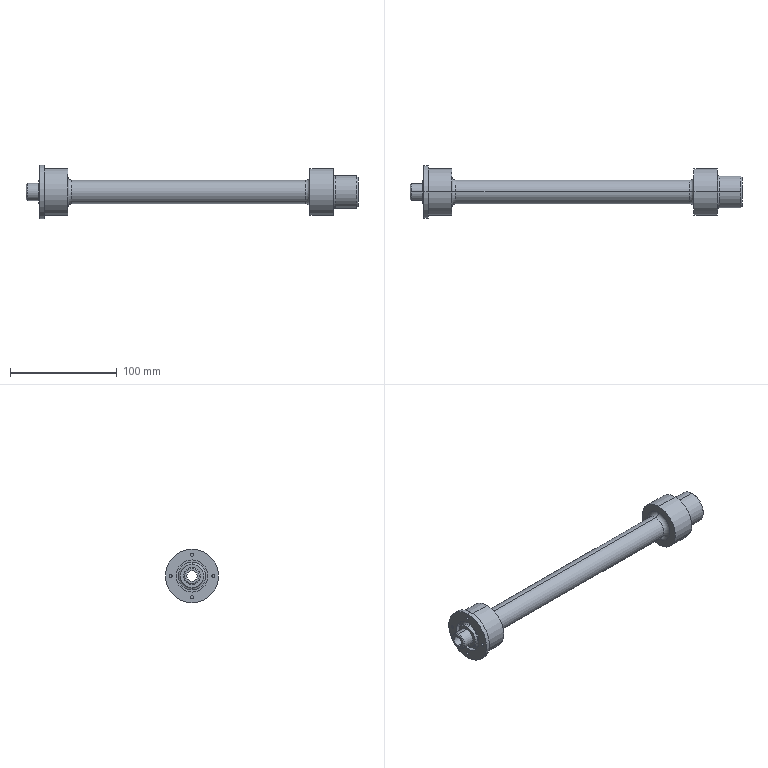Part | NX | features BREP 1 | 1 solid | 51 faces | box 311 x 50 x 50 mm | volume 154727 mm3 | cylinder 26 | plane 13 | torus 8 | cone 4 | commonest cylinder face diameters 3 x8 22 x4 30 x4 44 x4 10 x2 16 x2
STEP:
#1=CARTESIAN_POINT('',(-39.144,0.,21.5));
#2=VERTEX_POINT('',#1);
#3=CARTESIAN_POINT('',(-39.144,0.,18.5));
#4=VERTEX_POINT('',#3);
#5=CARTESIAN_POINT('',(-39.144,0.,20.));
#6=DIRECTION('',(1.,0.,0.));
#7=DIRECTION('',(0.,0.,-1.));
#8=AXIS2_PLACEMENT_3D('',#5,#6,#7);
#9=CIRCLE('',#8,1.5);
#10=EDGE_CURVE('',#2,#4,#9,.T.);
#11=ORIENTED_EDGE('',*,*,#10,.F.);
#12=CARTESIAN_POINT('',(-31.144,0.,21.5));
#13=VERTEX_POINT('',#12);
#14=CARTESIAN_POINT('',(-39.144,0.,21.5));
#15=DIRECTION('',(1.,0.,0.));
#16=VECTOR('',#15,1000.);
#17=LINE('',#14,#16);
#18=EDGE_CURVE('',#13,#2,#17,.F.);
#19=ORIENTED_EDGE('',*,*,#18,.F.);
#20=CARTESIAN_POINT('',(-31.144,0.,18.5));
#21=VERTEX_POINT('',#20);
#22=CARTESIAN_POINT('',(-31.144,0.,20.));
#23=DIRECTION('',(1.,0.,0.));
#24=DIRECTION('',(0.,0.,-1.));
#25=AXIS2_PLACEMENT_3D('',#22,#23,#24);
#26=CIRCLE('',#25,1.5);
#27=EDGE_CURVE('',#13,#21,#26,.T.);
#28=ORIENTED_EDGE('',*,*,#27,.T.);
#29=CARTESIAN_POINT('',(-39.144,0.,18.5));
#30=DIRECTION('',(1.,0.,0.));
#31=VECTOR('',#30,1000.);
#32=LINE('',#29,#31);
#33=EDGE_CURVE('',#21,#4,#32,.F.);
#34=ORIENTED_EDGE('',*,*,#33,.T.);
#35=EDGE_LOOP('',(#11,#19,#28,#34));
#36=FACE_BOUND('',#35,.T.);
#37=CARTESIAN_POINT('',(-39.144,0.,20.));
#38=DIRECTION('',(1.,0.,0.));
#39=DIRECTION('',(0.,0.,1.));
#40=AXIS2_PLACEMENT_3D('',#37,#38,#39);
#41=CYLINDRICAL_SURFACE('',#40,1.5);
#42=ADVANCED_FACE('',(#36),#41,.F.);
#43=CARTESIAN_POINT('',(-39.144,-20.,1.5));
#44=VERTEX_POINT('',#43);
#45=CARTESIAN_POINT('',(-39.144,-20.,-1.5));
#46=VERTEX_POINT('',#45);
#47=CARTESIAN_POINT('',(-39.144,-20.,0.));
#48=DIRECTION('',(1.,0.,0.));
#49=DIRECTION('',(0.,0.,-1.));
#50=AXIS2_PLACEMENT_3D('',#47,#48,#49);
#51=CIRCLE('',#50,1.5);
#52=EDGE_CURVE('',#44,#46,#51,.T.);
#53=ORIENTED_EDGE('',*,*,#52,.F.);
#54=CARTESIAN_POINT('',(-31.144,-20.,1.5));
#55=VERTEX_POINT('',#54);
#56=CARTESIAN_POINT('',(-39.144,-20.,1.5));
#57=DIRECTION('',(1.,0.,0.));
#58=VECTOR('',#57,1000.);
#59=LINE('',#56,#58);
#60=EDGE_CURVE('',#55,#44,#59,.F.);
#61=ORIENTED_EDGE('',*,*,#60,.F.);
#62=CARTESIAN_POINT('',(-31.144,-20.,-1.5));
#63=VERTEX_POINT('',#62);
#64=CARTESIAN_POINT('',(-31.144,-20.,0.));
#65=DIRECTION('',(1.,0.,0.));
#66=DIRECTION('',(0.,0.,-1.));
#67=AXIS2_PLACEMENT_3D('',#64,#65,#66);
#68=CIRCLE('',#67,1.5);
#69=EDGE_CURVE('',#55,#63,#68,.T.);
#70=ORIENTED_EDGE('',*,*,#69,.T.);
#71=CARTESIAN_POINT('',(-39.144,-20.,-1.5));
#72=DIRECTION('',(1.,0.,0.));
#73=VECTOR('',#72,1000.);
#74=LINE('',#71,#73);
#75=EDGE_CURVE('',#63,#46,#74,.F.);
#76=ORIENTED_EDGE('',*,*,#75,.T.);
#77=EDGE_LOOP('',(#53,#61,#70,#76));
#78=FACE_BOUND('',#77,.T.);
#79=CARTESIAN_POINT('',(-39.144,-20.,0.));
#80=DIRECTION('',(1.,0.,0.));
#81=DIRECTION('',(0.,0.,1.));
#82=AXIS2_PLACEMENT_3D('',#79,#80,#81);
#83=CYLINDRICAL_SURFACE('',#82,1.5);
#84=ADVANCED_FACE('',(#78),#83,.F.);
#85=CARTESIAN_POINT('',(-39.144,0.,-18.5));
#86=VERTEX_POINT('',#85);
#87=CARTESIAN_POINT('',(-39.144,0.,-21.5));
#88=VERTEX_POINT('',#87);
#89=CARTESIAN_POINT('',(-39.144,0.,-20.));
#90=DIRECTION('',(1.,0.,0.));
#91=DIRECTION('',(0.,0.,-1.));
#92=AXIS2_PLACEMENT_3D('',#89,#90,#91);
#93=CIRCLE('',#92,1.5);
#94=EDGE_CURVE('',#86,#88,#93,.T.);
#95=ORIENTED_EDGE('',*,*,#94,.F.);
#96=CARTESIAN_POINT('',(-31.144,0.,-18.5));
#97=VERTEX_POINT('',#96);
#98=CARTESIAN_POINT('',(-39.144,0.,-18.5));
#99=DIRECTION('',(1.,0.,0.));
#100=VECTOR('',#99,1000.);
#101=LINE('',#98,#100);
#102=EDGE_CURVE('',#97,#86,#101,.F.);
#103=ORIENTED_EDGE('',*,*,#102,.F.);
#104=CARTESIAN_POINT('',(-31.144,0.,-21.5));
#105=VERTEX_POINT('',#104);
#106=CARTESIAN_POINT('',(-31.144,0.,-20.));
#107=DIRECTION('',(1.,0.,0.));
#108=DIRECTION('',(0.,0.,-1.));
#109=AXIS2_PLACEMENT_3D('',#106,#107,#108);
#110=CIRCLE('',#109,1.5);
#111=EDGE_CURVE('',#97,#105,#110,.T.);
#112=ORIENTED_EDGE('',*,*,#111,.T.);
#113=CARTESIAN_POINT('',(-39.144,0.,-21.5));
#114=DIRECTION('',(1.,0.,0.));
#115=VECTOR('',#114,1000.);
#116=LINE('',#113,#115);
#117=EDGE_CURVE('',#105,#88,#116,.F.);
#118=ORIENTED_EDGE('',*,*,#117,.T.);
#119=EDGE_LOOP('',(#95,#103,#112,#118));
#120=FACE_BOUND('',#119,.T.);
#121=CARTESIAN_POINT('',(-39.144,0.,-20.));
#122=DIRECTION('',(1.,0.,0.));
#123=DIRECTION('',(0.,0.,1.));
#124=AXIS2_PLACEMENT_3D('',#121,#122,#123);
#125=CYLINDRICAL_SURFACE('',#124,1.5);
#126=ADVANCED_FACE('',(#120),#125,.F.);
#127=CARTESIAN_POINT('',(-39.144,20.,1.5));
#128=VERTEX_POINT('',#127);
#129=CARTESIAN_POINT('',(-39.144,20.,-1.5));
#130=VERTEX_POINT('',#129);
#131=CARTESIAN_POINT('',(-39.144,20.,0.));
#132=DIRECTION('',(1.,0.,0.));
#133=DIRECTION('',(0.,0.,-1.));
#134=AXIS2_PLACEMENT_3D('',#131,#132,#133);
#135=CIRCLE('',#134,1.5);
#136=EDGE_CURVE('',#128,#130,#135,.T.);
#137=ORIENTED_EDGE('',*,*,#136,.F.);
#138=CARTESIAN_POINT('',(-31.144,20.,1.5));
#139=VERTEX_POINT('',#138);
#140=CARTESIAN_POINT('',(-39.144,20.,1.5));
#141=DIRECTION('',(1.,0.,0.));
#142=VECTOR('',#141,1000.);
#143=LINE('',#140,#142);
#144=EDGE_CURVE('',#139,#128,#143,.F.);
#145=ORIENTED_EDGE('',*,*,#144,.F.);
#146=CARTESIAN_POINT('',(-31.144,20.,-1.5));
#147=VERTEX_POINT('',#146);
#148=CARTESIAN_POINT('',(-31.144,20.,0.));
#149=DIRECTION('',(1.,0.,0.));
#150=DIRECTION('',(0.,0.,-1.));
#151=AXIS2_PLACEMENT_3D('',#148,#149,#150);
#152=CIRCLE('',#151,1.5);
#153=EDGE_CURVE('',#139,#147,#152,.T.);
#154=ORIENTED_EDGE('',*,*,#153,.T.);
#155=CARTESIAN_POINT('',(-39.144,20.,-1.5));
#156=DIRECTION('',(1.,0.,0.));
#157=VECTOR('',#156,1000.);
#158=LINE('',#155,#157);
#159=EDGE_CURVE('',#147,#130,#158,.F.);
#160=ORIENTED_EDGE('',*,*,#159,.T.);
#161=EDGE_LOOP('',(#137,#145,#154,#160));
#162=FACE_BOUND('',#161,.T.);
#163=CARTESIAN_POINT('',(-39.144,20.,0.));
#164=DIRECTION('',(1.,0.,0.));
#165=DIRECTION('',(0.,0.,1.));
#166=AXIS2_PLACEMENT_3D('',#163,#164,#165);
#167=CYLINDRICAL_SURFACE('',#166,1.5);
#168=ADVANCED_FACE('',(#162),#167,.F.);
#169=CARTESIAN_POINT('',(-39.144,0.,-15.));
#170=VERTEX_POINT('',#169);
#171=CARTESIAN_POINT('',(-39.144,0.,15.));
#172=VERTEX_POINT('',#171);
#173=CARTESIAN_POINT('',(-39.144,0.,0.));
#174=DIRECTION('',(-1.,0.,0.));
#175=DIRECTION('',(0.,0.,1.));
#176=AXIS2_PLACEMENT_3D('',#173,#174,#175);
#177=CIRCLE('',#176,15.);
#178=EDGE_CURVE('',#170,#172,#177,.T.);
#179=ORIENTED_EDGE('',*,*,#178,.T.);
#180=CARTESIAN_POINT('',(-35.144,0.,15.));
#181=VERTEX_POINT('',#180);
#182=CARTESIAN_POINT('',(-39.144,0.,15.));
#183=DIRECTION('',(1.,0.,0.));
#184=VECTOR('',#183,1000.);
#185=LINE('',#182,#184);
#186=EDGE_CURVE('',#181,#172,#185,.F.);
#187=ORIENTED_EDGE('',*,*,#186,.F.);
#188=CARTESIAN_POINT('',(-35.144,0.,-15.));
#189=VERTEX_POINT('',#188);
#190=CARTESIAN_POINT('',(-35.144,0.,0.));
#191=DIRECTION('',(-1.,0.,0.));
#192=DIRECTION('',(0.,0.,1.));
#193=AXIS2_PLACEMENT_3D('',#190,#191,#192);
#194=CIRCLE('',#193,15.);
#195=EDGE_CURVE('',#189,#181,#194,.T.);
#196=ORIENTED_EDGE('',*,*,#195,.F.);
#197=CARTESIAN_POINT('',(-39.144,0.,-15.));
#198=DIRECTION('',(1.,0.,0.));
#199=VECTOR('',#198,1000.);
#200=LINE('',#197,#199);
#201=EDGE_CURVE('',#189,#170,#200,.F.);
#202=ORIENTED_EDGE('',*,*,#201,.T.);
#203=EDGE_LOOP('',(#179,#187,#196,#202));
#204=FACE_BOUND('',#203,.T.);
#205=CARTESIAN_POINT('',(-39.144,0.,0.));
#206=DIRECTION('',(1.,0.,0.));
#207=DIRECTION('',(0.,0.,1.));
#208=AXIS2_PLACEMENT_3D('',#205,#206,#207);
#209=CYLINDRICAL_SURFACE('',#208,15.);
#210=ADVANCED_FACE('',(#204),#209,.F.);
#211=CARTESIAN_POINT('',(-39.144,0.,25.));
#212=VERTEX_POINT('',#211);
#213=CARTESIAN_POINT('',(-39.144,0.,-25.));
#214=VERTEX_POINT('',#213);
#215=CARTESIAN_POINT('',(-39.144,0.,0.));
#216=DIRECTION('',(-1.,0.,0.));
#217=DIRECTION('',(0.,0.,1.));
#218=AXIS2_PLACEMENT_3D('',#215,#216,#217);
#219=CIRCLE('',#218,25.);
#220=EDGE_CURVE('',#212,#214,#219,.T.);
#221=ORIENTED_EDGE('',*,*,#220,.F.);
#222=CARTESIAN_POINT('',(-35.144,0.,25.));
#223=VERTEX_POINT('',#222);
#224=CARTESIAN_POINT('',(-39.144,0.,25.));
#225=DIRECTION('',(1.,0.,0.));
#226=VECTOR('',#225,1000.);
#227=LINE('',#224,#226);
#228=EDGE_CURVE('',#223,#212,#227,.F.);
#229=ORIENTED_EDGE('',*,*,#228,.F.);
#230=CARTESIAN_POINT('',(-35.144,0.,-25.));
#231=VERTEX_POINT('',#230);
#232=CARTESIAN_POINT('',(-35.144,0.,0.));
#233=DIRECTION('',(-1.,0.,0.));
#234=DIRECTION('',(0.,0.,1.));
#235=AXIS2_PLACEMENT_3D('',#232,#233,#234);
#236=CIRCLE('',#235,25.);
#237=EDGE_CURVE('',#223,#231,#236,.T.);
#238=ORIENTED_EDGE('',*,*,#237,.T.);
#239=CARTESIAN_POINT('',(-39.144,0.,-25.));
#240=DIRECTION('',(1.,0.,0.));
#241=VECTOR('',#240,1000.);
#242=LINE('',#239,#241);
#243=EDGE_CURVE('',#231,#214,#242,.F.);
#244=ORIENTED_EDGE('',*,*,#243,.T.);
#245=EDGE_LOOP('',(#221,#229,#238,#244));
#246=FACE_BOUND('',#245,.T.);
#247=CARTESIAN_POINT('',(-39.144,0.,0.));
#248=DIRECTION('',(1.,0.,0.));
#249=DIRECTION('',(0.,0.,1.));
#250=AXIS2_PLACEMENT_3D('',#247,#248,#249);
#251=CYLINDRICAL_SURFACE('',#250,25.);
#252=ADVANCED_FACE('',(#246),#251,.T.);
#253=CARTESIAN_POINT('',(-13.144,0.,22.));
#254=VERTEX_POINT('',#253);
#255=CARTESIAN_POINT('',(-13.144,0.,-22.));
#256=VERTEX_POINT('',#255);
#257=CARTESIAN_POINT('',(-13.144,0.,0.));
#258=DIRECTION('',(-1.,0.,0.));
#259=DIRECTION('',(0.,0.,1.));
#260=AXIS2_PLACEMENT_3D('',#257,#258,#259);
#261=CIRCLE('',#260,22.);
#262=EDGE_CURVE('',#254,#256,#261,.T.);
#263=ORIENTED_EDGE('',*,*,#262,.T.);
#264=CARTESIAN_POINT('',(-35.144,0.,-22.));
#265=VERTEX_POINT('',#264);
#266=CARTESIAN_POINT('',(-63.195,0.,-22.));
#267=DIRECTION('',(-1.,0.,0.));
#268=VECTOR('',#267,1000.);
#269=LINE('',#266,#268);
#270=EDGE_CURVE('',#256,#265,#269,.T.);
#271=ORIENTED_EDGE('',*,*,#270,.T.);
#272=CARTESIAN_POINT('',(-35.144,0.,22.));
#273=VERTEX_POINT('',#272);
#274=CARTESIAN_POINT('',(-35.144,0.,0.));
#275=DIRECTION('',(-1.,0.,0.));
#276=DIRECTION('',(0.,0.,1.));
#277=AXIS2_PLACEMENT_3D('',#274,#275,#276);
#278=CIRCLE('',#277,22.);
#279=EDGE_CURVE('',#273,#265,#278,.T.);
#280=ORIENTED_EDGE('',*,*,#279,.F.);
#281=CARTESIAN_POINT('',(-63.195,0.,22.));
#282=DIRECTION('',(-1.,0.,0.));
#283=VECTOR('',#282,1000.);
#284=LINE('',#281,#283);
#285=EDGE_CURVE('',#254,#273,#284,.T.);
#286=ORIENTED_EDGE('',*,*,#285,.F.);
#287=EDGE_LOOP('',(#263,#271,#280,#286));
#288=FACE_BOUND('',#287,.T.);
#289=CARTESIAN_POINT('',(-63.195,0.,0.));
#290=DIRECTION('',(-1.,0.,0.));
#291=DIRECTION('',(0.,0.,-1.));
#292=AXIS2_PLACEMENT_3D('',#289,#290,#291);
#293=CYLINDRICAL_SURFACE('',#292,22.);
#294=ADVANCED_FACE('',(#288),#293,.T.);
#295=CARTESIAN_POINT('',(-13.144,0.,-15.));
#296=VERTEX_POINT('',#295);
#297=CARTESIAN_POINT('',(-13.144,0.,15.));
#298=VERTEX_POINT('',#297);
#299=CARTESIAN_POINT('',(-13.144,0.,0.));
#300=DIRECTION('',(-1.,0.,0.));
#301=DIRECTION('',(0.,0.,1.));
#302=AXIS2_PLACEMENT_3D('',#299,#300,#301);
#303=CIRCLE('',#302,15.);
#304=EDGE_CURVE('',#296,#298,#303,.T.);
#305=ORIENTED_EDGE('',*,*,#304,.F.);
#306=CARTESIAN_POINT('',(-9.144,0.,-11.));
#307=VERTEX_POINT('',#306);
#308=CARTESIAN_POINT('',(-9.144,0.,-15.));
#309=DIRECTION('',(0.,1.,0.));
#310=DIRECTION('',(0.,0.,1.));
#311=AXIS2_PLACEMENT_3D('',#308,#309,#310);
#312=CIRCLE('',#311,4.);
#313=EDGE_CURVE('',#296,#307,#312,.T.);
#314=ORIENTED_EDGE('',*,*,#313,.T.);
#315=CARTESIAN_POINT('',(-9.144,0.,11.));
#316=VERTEX_POINT('',#315);
#317=CARTESIAN_POINT('',(-9.144,0.,0.));
#318=DIRECTION('',(-1.,0.,0.));
#319=DIRECTION('',(0.,0.,1.));
#320=AXIS2_PLACEMENT_3D('',#317,#318,#319);
#321=CIRCLE('',#320,11.);
#322=EDGE_CURVE('',#307,#316,#321,.T.);
#323=ORIENTED_EDGE('',*,*,#322,.T.);
#324=CARTESIAN_POINT('',(-9.144,0.,15.));
#325=DIRECTION('',(0.,-1.,0.));
#326=DIRECTION('',(1.,0.,0.));
#327=AXIS2_PLACEMENT_3D('',#324,#325,#326);
#328=CIRCLE('',#327,4.);
#329=EDGE_CURVE('',#298,#316,#328,.T.);
#330=ORIENTED_EDGE('',*,*,#329,.F.);
#331=EDGE_LOOP('',(#305,#314,#323,#330));
#332=FACE_BOUND('',#331,.T.);
#333=CARTESIAN_POINT('',(-9.144,0.,0.));
#334=DIRECTION('',(-1.,0.,0.));
#335=DIRECTION('',(0.,0.,-1.));
#336=AXIS2_PLACEMENT_3D('',#333,#334,#335);
#337=TOROIDAL_SURFACE('',#336,15.,4.);
#338=ADVANCED_FACE('',(#332),#337,.F.);
#339=CARTESIAN_POINT('',(209.856,0.,11.));
#340=VERTEX_POINT('',#339);
#341=CARTESIAN_POINT('',(209.856,0.,-11.));
#342=VERTEX_POINT('',#341);
#343=CARTESIAN_POINT('',(209.856,0.,0.));
#344=DIRECTION('',(-1.,0.,0.));
#345=DIRECTION('',(0.,0.,1.));
#346=AXIS2_PLACEMENT_3D('',#343,#344,#345);
#347=CIRCLE('',#346,11.);
#348=EDGE_CURVE('',#340,#342,#347,.T.);
#349=ORIENTED_EDGE('',*,*,#348,.T.);
#350=CARTESIAN_POINT('',(-63.195,0.,-11.));
#351=DIRECTION('',(-1.,0.,0.));
#352=VECTOR('',#351,1000.);
#353=LINE('',#350,#352);
#354=EDGE_CURVE('',#342,#307,#353,.T.);
#355=ORIENTED_EDGE('',*,*,#354,.T.);
#356=CARTESIAN_POINT('',(-9.144,0.,0.));
#357=DIRECTION('',(-1.,0.,0.));
#358=DIRECTION('',(0.,0.,1.));
#359=AXIS2_PLACEMENT_3D('',#356,#357,#358);
#360=CIRCLE('',#359,11.);
#361=EDGE_CURVE('',#316,#307,#360,.T.);
#362=ORIENTED_EDGE('',*,*,#361,.F.);
#363=CARTESIAN_POINT('',(-63.195,0.,11.));
#364=DIRECTION('',(-1.,0.,0.));
#365=VECTOR('',#364,1000.);
#366=LINE('',#363,#365);
#367=EDGE_CURVE('',#340,#316,#366,.T.);
#368=ORIENTED_EDGE('',*,*,#367,.F.);
#369=EDGE_LOOP('',(#349,#355,#362,#368));
#370=FACE_BOUND('',#369,.T.);
#371=CARTESIAN_POINT('',(-63.195,0.,0.));
#372=DIRECTION('',(-1.,0.,0.));
#373=DIRECTION('',(0.,0.,-1.));
#374=AXIS2_PLACEMENT_3D('',#371,#372,#373);
#375=CYLINDRICAL_SURFACE('',#374,11.);
#376=ADVANCED_FACE('',(#370),#375,.T.);
#377=CARTESIAN_POINT('',(209.856,0.,0.));
#378=DIRECTION('',(-1.,0.,0.));
#379=DIRECTION('',(0.,0.,1.));
#380=AXIS2_PLACEMENT_3D('',#377,#378,#379);
#381=CIRCLE('',#380,11.);
#382=EDGE_CURVE('',#342,#340,#381,.T.);
#383=ORIENTED_EDGE('',*,*,#382,.F.);
#384=CARTESIAN_POINT('',(213.856,0.,-15.));
#385=VERTEX_POINT('',#384);
#386=CARTESIAN_POINT('',(209.856,0.,-15.));
#387=DIRECTION('',(0.,1.,0.));
#388=DIRECTION('',(0.,0.,1.));
#389=AXIS2_PLACEMENT_3D('',#386,#387,#388);
#390=CIRCLE('',#389,4.);
#391=EDGE_CURVE('',#342,#385,#390,.T.);
#392=ORIENTED_EDGE('',*,*,#391,.T.);
#393=CARTESIAN_POINT('',(213.856,0.,15.));
#394=VERTEX_POINT('',#393);
#395=CARTESIAN_POINT('',(213.856,0.,0.));
#396=DIRECTION('',(-1.,0.,0.));
#397=DIRECTION('',(0.,0.,1.));
#398=AXIS2_PLACEMENT_3D('',#395,#396,#397);
#399=CIRCLE('',#398,15.);
#400=EDGE_CURVE('',#385,#394,#399,.T.);
#401=ORIENTED_EDGE('',*,*,#400,.T.);
#402=CARTESIAN_POINT('',(209.856,0.,15.));
#403=DIRECTION('',(0.,-1.,0.));
#404=DIRECTION('',(1.,0.,0.));
#405=AXIS2_PLACEMENT_3D('',#402,#403,#404);
#406=CIRCLE('',#405,4.);
#407=EDGE_CURVE('',#340,#394,#406,.T.);
#408=ORIENTED_EDGE('',*,*,#407,.F.);
#409=EDGE_LOOP('',(#383,#392,#401,#408));
#410=FACE_BOUND('',#409,.T.);
#411=CARTESIAN_POINT('',(209.856,0.,0.));
#412=DIRECTION('',(-1.,0.,0.));
#413=DIRECTION('',(0.,0.,-1.));
#414=AXIS2_PLACEMENT_3D('',#411,#412,#413);
#415=TOROIDAL_SURFACE('',#414,15.,4.);
#416=ADVANCED_FACE('',(#410),#415,.F.);
#417=CARTESIAN_POINT('',(235.856,0.,22.));
#418=VERTEX_POINT('',#417);
#419=CARTESIAN_POINT('',(235.856,0.,-22.));
#420=VERTEX_POINT('',#419);
#421=CARTESIAN_POINT('',(235.856,0.,0.));
#422=DIRECTION('',(-1.,0.,0.));
#423=DIRECTION('',(0.,0.,1.));
#424=AXIS2_PLACEMENT_3D('',#421,#422,#423);
#425=CIRCLE('',#424,22.);
#426=EDGE_CURVE('',#418,#420,#425,.T.);
#427=ORIENTED_EDGE('',*,*,#426,.T.);
#428=CARTESIAN_POINT('',(213.856,0.,-22.));
#429=VERTEX_POINT('',#428);
#430=CARTESIAN_POINT('',(-63.195,0.,-22.));
#431=DIRECTION('',(-1.,0.,0.));
#432=VECTOR('',#431,1000.);
#433=LINE('',#430,#432);
#434=EDGE_CURVE('',#420,#429,#433,.T.);
#435=ORIENTED_EDGE('',*,*,#434,.T.);
#436=CARTESIAN_POINT('',(213.856,0.,22.));
#437=VERTEX_POINT('',#436);
#438=CARTESIAN_POINT('',(213.856,0.,0.));
#439=DIRECTION('',(-1.,0.,0.));
#440=DIRECTION('',(0.,0.,1.));
#441=AXIS2_PLACEMENT_3D('',#438,#439,#440);
#442=CIRCLE('',#441,22.);
#443=EDGE_CURVE('',#437,#429,#442,.T.);
#444=ORIENTED_EDGE('',*,*,#443,.F.);
#445=CARTESIAN_POINT('',(-63.195,0.,22.));
#446=DIRECTION('',(-1.,0.,0.));
#447=VECTOR('',#446,1000.);
#448=LINE('',#445,#447);
#449=EDGE_CURVE('',#418,#437,#448,.T.);
#450=ORIENTED_EDGE('',*,*,#449,.F.);
#451=EDGE_LOOP('',(#427,#435,#444,#450));
#452=FACE_BOUND('',#451,.T.);
#453=CARTESIAN_POINT('',(-63.195,0.,0.));
#454=DIRECTION('',(-1.,0.,0.));
#455=DIRECTION('',(0.,0.,-1.));
#456=AXIS2_PLACEMENT_3D('',#453,#454,#455);
#457=CYLINDRICAL_SURFACE('',#456,22.);
#458=ADVANCED_FACE('',(#452),#457,.T.);
#459=CARTESIAN_POINT('',(235.856,0.,-17.));
#460=VERTEX_POINT('',#459);
#461=CARTESIAN_POINT('',(235.856,0.,17.));
#462=VERTEX_POINT('',#461);
#463=CARTESIAN_POINT('',(235.856,0.,0.));
#464=DIRECTION('',(-1.,0.,0.));
#465=DIRECTION('',(0.,0.,1.));
#466=AXIS2_PLACEMENT_3D('',#463,#464,#465);
#467=CIRCLE('',#466,17.);
#468=EDGE_CURVE('',#460,#462,#467,.T.);
#469=ORIENTED_EDGE('',*,*,#468,.F.);
#470=CARTESIAN_POINT('',(237.856,0.,-15.));
#471=VERTEX_POINT('',#470);
#472=CARTESIAN_POINT('',(237.856,0.,-17.));
#473=DIRECTION('',(0.,1.,0.));
#474=DIRECTION('',(0.,0.,1.));
#475=AXIS2_PLACEMENT_3D('',#472,#473,#474);
#476=CIRCLE('',#475,2.);
#477=EDGE_CURVE('',#460,#471,#476,.T.);
#478=ORIENTED_EDGE('',*,*,#477,.T.);
#479=CARTESIAN_POINT('',(237.856,0.,15.));
#480=VERTEX_POINT('',#479);
#481=CARTESIAN_POINT('',(237.856,0.,0.));
#482=DIRECTION('',(-1.,0.,0.));
#483=DIRECTION('',(0.,0.,1.));
#484=AXIS2_PLACEMENT_3D('',#481,#482,#483);
#485=CIRCLE('',#484,15.);
#486=EDGE_CURVE('',#471,#480,#485,.T.);
#487=ORIENTED_EDGE('',*,*,#486,.T.);
#488=CARTESIAN_POINT('',(237.856,0.,17.));
#489=DIRECTION('',(0.,-1.,0.));
#490=DIRECTION('',(1.,0.,0.));
#491=AXIS2_PLACEMENT_3D('',#488,#489,#490);
#492=CIRCLE('',#491,2.);
#493=EDGE_CURVE('',#462,#480,#492,.T.);
#494=ORIENTED_EDGE('',*,*,#493,.F.);
#495=EDGE_LOOP('',(#469,#478,#487,#494));
#496=FACE_BOUND('',#495,.T.);
#497=CARTESIAN_POINT('',(237.856,0.,0.));
#498=DIRECTION('',(-1.,0.,0.));
#499=DIRECTION('',(0.,0.,-1.));
#500=AXIS2_PLACEMENT_3D('',#497,#498,#499);
#501=TOROIDAL_SURFACE('',#500,17.,2.);
#502=ADVANCED_FACE('',(#496),#501,.F.);
#503=CARTESIAN_POINT('',(257.856,0.,15.));
#504=VERTEX_POINT('',#503);
#505=CARTESIAN_POINT('',(257.856,0.,-15.));
#506=VERTEX_POINT('',#505);
#507=CARTESIAN_POINT('',(257.856,0.,0.));
#508=DIRECTION('',(-1.,0.,0.));
#509=DIRECTION('',(0.,0.,1.));
#510=AXIS2_PLACEMENT_3D('',#507,#508,#509);
#511=CIRCLE('',#510,15.);
#512=EDGE_CURVE('',#504,#506,#511,.T.);
#513=ORIENTED_EDGE('',*,*,#512,.T.);
#514=CARTESIAN_POINT('',(-63.195,0.,-15.));
#515=DIRECTION('',(-1.,0.,0.));
#516=VECTOR('',#515,1000.);
#517=LINE('',#514,#516);
#518=EDGE_CURVE('',#506,#471,#517,.T.);
#519=ORIENTED_EDGE('',*,*,#518,.T.);
#520=CARTESIAN_POINT('',(237.856,0.,0.));
#521=DIRECTION('',(-1.,0.,0.));
#522=DIRECTION('',(0.,0.,1.));
#523=AXIS2_PLACEMENT_3D('',#520,#521,#522);
#524=CIRCLE('',#523,15.);
#525=EDGE_CURVE('',#480,#471,#524,.T.);
#526=ORIENTED_EDGE('',*,*,#525,.F.);
#527=CARTESIAN_POINT('',(-63.195,0.,15.));
#528=DIRECTION('',(-1.,0.,0.));
#529=VECTOR('',#528,1000.);
#530=LINE('',#527,#529);
#531=EDGE_CURVE('',#504,#480,#530,.T.);
#532=ORIENTED_EDGE('',*,*,#531,.F.);
#533=EDGE_LOOP('',(#513,#519,#526,#532));
#534=FACE_BOUND('',#533,.T.);
#535=CARTESIAN_POINT('',(-63.195,0.,0.));
#536=DIRECTION('',(-1.,0.,0.));
#537=DIRECTION('',(0.,0.,-1.));
#538=AXIS2_PLACEMENT_3D('',#535,#536,#537);
#539=CYLINDRICAL_SURFACE('',#538,15.);
#540=ADVANCED_FACE('',(#534),#539,.T.);
#541=CARTESIAN_POINT('',(258.856,0.,14.));
#542=VERTEX_POINT('',#541);
#543=CARTESIAN_POINT('',(258.856,0.,-14.));
#544=VERTEX_POINT('',#543);
#545=CARTESIAN_POINT('',(258.856,0.,0.));
#546=DIRECTION('',(-1.,0.,0.));
#547=DIRECTION('',(0.,0.,1.));
#548=AXIS2_PLACEMENT_3D('',#545,#546,#547);
#549=CIRCLE('',#548,14.);
#550=EDGE_CURVE('',#542,#544,#549,.T.);
#551=ORIENTED_EDGE('',*,*,#550,.T.);
#552=CARTESIAN_POINT('',(258.856,0.,-14.));
#553=DIRECTION('',(-0.7071,0.,-0.7071));
#554=VECTOR('',#553,1000.);
#555=LINE('',#552,#554);
#556=EDGE_CURVE('',#544,#506,#555,.T.);
#557=ORIENTED_EDGE('',*,*,#556,.T.);
#558=ORIENTED_EDGE('',*,*,#512,.F.);
#559=CARTESIAN_POINT('',(258.856,0.,14.));
#560=DIRECTION('',(-0.7071,0.,0.7071));
#561=VECTOR('',#560,1000.);
#562=LINE('',#559,#561);
#563=EDGE_CURVE('',#542,#504,#562,.T.);
#564=ORIENTED_EDGE('',*,*,#563,.F.);
#565=EDGE_LOOP('',(#551,#557,#558,#564));
#566=FACE_BOUND('',#565,.T.);
#567=CARTESIAN_POINT('',(258.856,0.,0.));
#568=DIRECTION('',(-1.,0.,0.));
#569=DIRECTION('',(0.,0.,-1.));
#570=AXIS2_PLACEMENT_3D('',#567,#568,#569);
#571=CONICAL_SURFACE('',#570,14.,0.7854);
#572=ADVANCED_FACE('',(#566),#571,.T.);
#573=CARTESIAN_POINT('',(258.856,0.,-5.));
#574=VERTEX_POINT('',#573);
#575=CARTESIAN_POINT('',(258.856,0.,5.));
#576=VERTEX_POINT('',#575);
#577=CARTESIAN_POINT('',(258.856,0.,0.));
#578=DIRECTION('',(-1.,0.,0.));
#579=DIRECTION('',(0.,0.,1.));
#580=AXIS2_PLACEMENT_3D('',#577,#578,#579);
#581=CIRCLE('',#580,5.);
#582=EDGE_CURVE('',#574,#576,#581,.T.);
#583=ORIENTED_EDGE('',*,*,#582,.F.);
#584=CARTESIAN_POINT('',(-52.144,0.,-5.));
#585=VERTEX_POINT('',#584);
#586=CARTESIAN_POINT('',(-63.195,0.,-5.));
#587=DIRECTION('',(-1.,0.,0.));
#588=VECTOR('',#587,1000.);
#589=LINE('',#586,#588);
#590=EDGE_CURVE('',#574,#585,#589,.T.);
#591=ORIENTED_EDGE('',*,*,#590,.T.);
#592=CARTESIAN_POINT('',(-52.144,0.,5.));
#593=VERTEX_POINT('',#592);
#594=CARTESIAN_POINT('',(-52.144,0.,0.));
#595=DIRECTION('',(-1.,0.,0.));
#596=DIRECTION('',(0.,0.,1.));
#597=AXIS2_PLACEMENT_3D('',#594,#595,#596);
#598=CIRCLE('',#597,5.);
#599=EDGE_CURVE('',#585,#593,#598,.T.);
#600=ORIENTED_EDGE('',*,*,#599,.T.);
#601=CARTESIAN_POINT('',(-63.195,0.,5.));
#602=DIRECTION('',(-1.,0.,0.));
#603=VECTOR('',#602,1000.);
#604=LINE('',#601,#603);
#605=EDGE_CURVE('',#576,#593,#604,.T.);
#606=ORIENTED_EDGE('',*,*,#605,.F.);
#607=EDGE_LOOP('',(#583,#591,#600,#606));
#608=FACE_BOUND('',#607,.T.);
#609=CARTESIAN_POINT('',(-63.195,0.,0.));
#610=DIRECTION('',(-1.,0.,0.));
#611=DIRECTION('',(0.,0.,-1.));
#612=AXIS2_PLACEMENT_3D('',#609,#610,#611);
#613=CYLINDRICAL_SURFACE('',#612,5.);
#614=ADVANCED_FACE('',(#608),#613,.F.);
#615=CARTESIAN_POINT('',(-52.144,0.,7.));
#616=VERTEX_POINT('',#615);
#617=CARTESIAN_POINT('',(-52.144,0.,-7.));
#618=VERTEX_POINT('',#617);
#619=CARTESIAN_POINT('',(-52.144,0.,0.));
#620=DIRECTION('',(-1.,0.,0.));
#621=DIRECTION('',(0.,0.,1.));
#622=AXIS2_PLACEMENT_3D('',#619,#620,#621);
#623=CIRCLE('',#622,7.);
#624=EDGE_CURVE('',#616,#618,#623,.T.);
#625=ORIENTED_EDGE('',*,*,#624,.F.);
#626=CARTESIAN_POINT('',(-51.144,0.,8.));
#627=VERTEX_POINT('',#626);
#628=CARTESIAN_POINT('',(-51.144,0.,8.));
#629=DIRECTION('',(0.7071,0.,0.7071));
#630=VECTOR('',#629,1000.);
#631=LINE('',#628,#630);
#632=EDGE_CURVE('',#627,#616,#631,.F.);
#633=ORIENTED_EDGE('',*,*,#632,.F.);
#634=CARTESIAN_POINT('',(-51.144,0.,-8.));
#635=VERTEX_POINT('',#634);
#636=CARTESIAN_POINT('',(-51.144,0.,0.));
#637=DIRECTION('',(-1.,0.,0.));
#638=DIRECTION('',(0.,0.,1.));
#639=AXIS2_PLACEMENT_3D('',#636,#637,#638);
#640=CIRCLE('',#639,8.);
#641=EDGE_CURVE('',#627,#635,#640,.T.);
#642=ORIENTED_EDGE('',*,*,#641,.T.);
#643=CARTESIAN_POINT('',(-51.144,0.,-8.));
#644=DIRECTION('',(0.7071,0.,-0.7071));
#645=VECTOR('',#644,1000.);
#646=LINE('',#643,#645);
#647=EDGE_CURVE('',#635,#618,#646,.F.);
#648=ORIENTED_EDGE('',*,*,#647,.T.);
#649=EDGE_LOOP('',(#625,#633,#642,#648));
#650=FACE_BOUND('',#649,.T.);
#651=CARTESIAN_POINT('',(-51.144,0.,0.));
#652=DIRECTION('',(1.,0.,0.));
#653=DIRECTION('',(0.,0.,1.));
#654=AXIS2_PLACEMENT_3D('',#651,#652,#653);
#655=CONICAL_SURFACE('',#654,8.,0.7854);
#656=ADVANCED_FACE('',(#650),#655,.T.);
#657=CARTESIAN_POINT('',(-40.144,0.,8.));
#658=VERTEX_POINT('',#657);
#659=CARTESIAN_POINT('',(-40.144,0.,-8.));
#660=VERTEX_POINT('',#659);
#661=CARTESIAN_POINT('',(-40.144,0.,0.));
#662=DIRECTION('',(-1.,0.,0.));
#663=DIRECTION('',(0.,0.,1.));
#664=AXIS2_PLACEMENT_3D('',#661,#662,#663);
#665=CIRCLE('',#664,8.);
#666=EDGE_CURVE('',#658,#660,#665,.T.);
#667=ORIENTED_EDGE('',*,*,#666,.T.);
#668=CARTESIAN_POINT('',(-63.195,0.,-8.));
#669=DIRECTION('',(-1.,0.,0.));
#670=VECTOR('',#669,1000.);
#671=LINE('',#668,#670);
#672=EDGE_CURVE('',#660,#635,#671,.T.);
#673=ORIENTED_EDGE('',*,*,#672,.T.);
#674=ORIENTED_EDGE('',*,*,#641,.F.);
#675=CARTESIAN_POINT('',(-63.195,0.,8.));
#676=DIRECTION('',(-1.,0.,0.));
#677=VECTOR('',#676,1000.);
#678=LINE('',#675,#677);
#679=EDGE_CURVE('',#658,#627,#678,.T.);
#680=ORIENTED_EDGE('',*,*,#679,.F.);
#681=EDGE_LOOP('',(#667,#673,#674,#680));
#682=FACE_BOUND('',#681,.T.);
#683=CARTESIAN_POINT('',(-63.195,0.,0.));
#684=DIRECTION('',(-1.,0.,0.));
#685=DIRECTION('',(0.,0.,-1.));
#686=AXIS2_PLACEMENT_3D('',#683,#684,#685);
#687=CYLINDRICAL_SURFACE('',#686,8.);
#688=ADVANCED_FACE('',(#682),#687,.T.);
#689=CARTESIAN_POINT('',(-37.144,0.,11.));
#690=VERTEX_POINT('',#689);
#691=CARTESIAN_POINT('',(-37.144,0.,-11.));
#692=VERTEX_POINT('',#691);
#693=CARTESIAN_POINT('',(-37.144,0.,0.));
#694=DIRECTION('',(-1.,0.,0.));
#695=DIRECTION('',(0.,0.,1.));
#696=AXIS2_PLACEMENT_3D('',#693,#694,#695);
#697=CIRCLE('',#696,11.);
#698=EDGE_CURVE('',#690,#692,#697,.T.);
#699=ORIENTED_EDGE('',*,*,#698,.T.);
#700=CARTESIAN_POINT('',(-40.144,0.,-11.));
#701=VERTEX_POINT('',#700);
#702=CARTESIAN_POINT('',(-63.195,0.,-11.));
#703=DIRECTION('',(-1.,0.,0.));
#704=VECTOR('',#703,1000.);
#705=LINE('',#702,#704);
#706=EDGE_CURVE('',#692,#701,#705,.T.);
#707=ORIENTED_EDGE('',*,*,#706,.T.);
#708=CARTESIAN_POINT('',(-40.144,0.,11.));
#709=VERTEX_POINT('',#708);
#710=CARTESIAN_POINT('',(-40.144,0.,0.));
#711=DIRECTION('',(-1.,0.,0.));
#712=DIRECTION('',(0.,0.,1.));
#713=AXIS2_PLACEMENT_3D('',#710,#711,#712);
#714=CIRCLE('',#713,11.);
#715=EDGE_CURVE('',#709,#701,#714,.T.);
#716=ORIENTED_EDGE('',*,*,#715,.F.);
#717=CARTESIAN_POINT('',(-63.195,0.,11.));
#718=DIRECTION('',(-1.,0.,0.));
#719=VECTOR('',#718,1000.);
#720=LINE('',#717,#719);
#721=EDGE_CURVE('',#690,#709,#720,.T.);
#722=ORIENTED_EDGE('',*,*,#721,.F.);
#723=EDGE_LOOP('',(#699,#707,#716,#722));
#724=FACE_BOUND('',#723,.T.);
#725=CARTESIAN_POINT('',(-63.195,0.,0.));
#726=DIRECTION('',(-1.,0.,0.));
#727=DIRECTION('',(0.,0.,-1.));
#728=AXIS2_PLACEMENT_3D('',#725,#726,#727);
#729=CYLINDRICAL_SURFACE('',#728,11.);
#730=ADVANCED_FACE('',(#724),#729,.T.);
#731=CARTESIAN_POINT('',(-37.144,0.,0.));
#732=DIRECTION('',(-1.,0.,0.));
#733=DIRECTION('',(0.,0.,1.));
#734=AXIS2_PLACEMENT_3D('',#731,#732,#733);
#735=CIRCLE('',#734,11.);
#736=EDGE_CURVE('',#692,#690,#735,.T.);
#737=ORIENTED_EDGE('',*,*,#736,.F.);
#738=CARTESIAN_POINT('',(-35.144,0.,-13.));
#739=VERTEX_POINT('',#738);
#740=CARTESIAN_POINT('',(-37.144,0.,-13.));
#741=DIRECTION('',(0.,1.,0.));
#742=DIRECTION('',(0.,0.,1.));
#743=AXIS2_PLACEMENT_3D('',#740,#741,#742);
#744=CIRCLE('',#743,2.);
#745=EDGE_CURVE('',#692,#739,#744,.T.);
#746=ORIENTED_EDGE('',*,*,#745,.T.);
#747=CARTESIAN_POINT('',(-35.144,0.,13.));
#748=VERTEX_POINT('',#747);
#749=CARTESIAN_POINT('',(-35.144,0.,0.));
#750=DIRECTION('',(-1.,0.,0.));
#751=DIRECTION('',(0.,0.,1.));
#752=AXIS2_PLACEMENT_3D('',#749,#750,#751);
#753=CIRCLE('',#752,13.);
#754=EDGE_CURVE('',#739,#748,#753,.T.);
#755=ORIENTED_EDGE('',*,*,#754,.T.);
#756=CARTESIAN_POINT('',(-37.144,0.,13.));
#757=DIRECTION('',(0.,-1.,0.));
#758=DIRECTION('',(1.,0.,0.));
#759=AXIS2_PLACEMENT_3D('',#756,#757,#758);
#760=CIRCLE('',#759,2.);
#761=EDGE_CURVE('',#690,#748,#760,.T.);
#762=ORIENTED_EDGE('',*,*,#761,.F.);
#763=EDGE_LOOP('',(#737,#746,#755,#762));
#764=FACE_BOUND('',#763,.T.);
#765=CARTESIAN_POINT('',(-37.144,0.,0.));
#766=DIRECTION('',(-1.,0.,0.));
#767=DIRECTION('',(0.,0.,-1.));
#768=AXIS2_PLACEMENT_3D('',#765,#766,#767);
#769=TOROIDAL_SURFACE('',#768,13.,2.);
#770=ADVANCED_FACE('',(#764),#769,.F.);
#771=ORIENTED_EDGE('',*,*,#745,.F.);
#772=ORIENTED_EDGE('',*,*,#698,.F.);
#773=ORIENTED_EDGE('',*,*,#761,.T.);
#774=CARTESIAN_POINT('',(-35.144,0.,0.));
#775=DIRECTION('',(-1.,0.,0.));
#776=DIRECTION('',(0.,0.,1.));
#777=AXIS2_PLACEMENT_3D('',#774,#775,#776);
#778=CIRCLE('',#777,13.);
#779=EDGE_CURVE('',#748,#739,#778,.T.);
#780=ORIENTED_EDGE('',*,*,#779,.T.);
#781=EDGE_LOOP('',(#771,#772,#773,#780));
#782=FACE_BOUND('',#781,.T.);
#783=CARTESIAN_POINT('',(-37.144,0.,0.));
#784=DIRECTION('',(-1.,0.,0.));
#785=DIRECTION('',(0.,0.,-1.));
#786=AXIS2_PLACEMENT_3D('',#783,#784,#785);
#787=TOROIDAL_SURFACE('',#786,13.,2.);
#788=ADVANCED_FACE('',(#782),#787,.F.);
#789=ORIENTED_EDGE('',*,*,#706,.F.);
#790=ORIENTED_EDGE('',*,*,#736,.T.);
#791=ORIENTED_EDGE('',*,*,#721,.T.);
#792=CARTESIAN_POINT('',(-40.144,0.,0.));
#793=DIRECTION('',(-1.,0.,0.));
#794=DIRECTION('',(0.,0.,1.));
#795=AXIS2_PLACEMENT_3D('',#792,#793,#794);
#796=CIRCLE('',#795,11.);
#797=EDGE_CURVE('',#701,#709,#796,.T.);
#798=ORIENTED_EDGE('',*,*,#797,.F.);
#799=EDGE_LOOP('',(#789,#790,#791,#798));
#800=FACE_BOUND('',#799,.T.);
#801=CARTESIAN_POINT('',(-63.195,0.,0.));
#802=DIRECTION('',(-1.,0.,0.));
#803=DIRECTION('',(0.,0.,-1.));
#804=AXIS2_PLACEMENT_3D('',#801,#802,#803);
#805=CYLINDRICAL_SURFACE('',#804,11.);
#806=ADVANCED_FACE('',(#800),#805,.T.);
#807=ORIENTED_EDGE('',*,*,#715,.T.);
#808=ORIENTED_EDGE('',*,*,#797,.T.);
#809=EDGE_LOOP('',(#807,#808));
#810=FACE_BOUND('',#809,.T.);
#811=ORIENTED_EDGE('',*,*,#666,.F.);
#812=CARTESIAN_POINT('',(-40.144,0.,0.));
#813=DIRECTION('',(-1.,0.,0.));
#814=DIRECTION('',(0.,0.,1.));
#815=AXIS2_PLACEMENT_3D('',#812,#813,#814);
#816=CIRCLE('',#815,8.);
#817=EDGE_CURVE('',#660,#658,#816,.T.);
#818=ORIENTED_EDGE('',*,*,#817,.F.);
#819=EDGE_LOOP('',(#811,#818));
#820=FACE_BOUND('',#819,.T.);
#821=CARTESIAN_POINT('',(-40.144,8.,0.));
#822=DIRECTION('',(1.,0.,0.));
#823=DIRECTION('',(0.,-1.,0.));
#824=AXIS2_PLACEMENT_3D('',#821,#822,#823);
#825=PLANE('',#824);
#826=ADVANCED_FACE('',(#810,#820),#825,.F.);
#827=ORIENTED_EDGE('',*,*,#672,.F.);
#828=ORIENTED_EDGE('',*,*,#817,.T.);
#829=ORIENTED_EDGE('',*,*,#679,.T.);
#830=CARTESIAN_POINT('',(-51.144,0.,0.));
#831=DIRECTION('',(-1.,0.,0.));
#832=DIRECTION('',(0.,0.,1.));
#833=AXIS2_PLACEMENT_3D('',#830,#831,#832);
#834=CIRCLE('',#833,8.);
#835=EDGE_CURVE('',#635,#627,#834,.T.);
#836=ORIENTED_EDGE('',*,*,#835,.F.);
#837=EDGE_LOOP('',(#827,#828,#829,#836));
#838=FACE_BOUND('',#837,.T.);
#839=CARTESIAN_POINT('',(-63.195,0.,0.));
#840=DIRECTION('',(-1.,0.,0.));
#841=DIRECTION('',(0.,0.,-1.));
#842=AXIS2_PLACEMENT_3D('',#839,#840,#841);
#843=CYLINDRICAL_SURFACE('',#842,8.);
#844=ADVANCED_FACE('',(#838),#843,.T.);
#845=ORIENTED_EDGE('',*,*,#632,.T.);
#846=CARTESIAN_POINT('',(-52.144,0.,0.));
#847=DIRECTION('',(-1.,0.,0.));
#848=DIRECTION('',(0.,0.,1.));
#849=AXIS2_PLACEMENT_3D('',#846,#847,#848);
#850=CIRCLE('',#849,7.);
#851=EDGE_CURVE('',#618,#616,#850,.T.);
#852=ORIENTED_EDGE('',*,*,#851,.F.);
#853=ORIENTED_EDGE('',*,*,#647,.F.);
#854=ORIENTED_EDGE('',*,*,#835,.T.);
#855=EDGE_LOOP('',(#845,#852,#853,#854));
#856=FACE_BOUND('',#855,.T.);
#857=CARTESIAN_POINT('',(-51.144,0.,0.));
#858=DIRECTION('',(1.,0.,0.));
#859=DIRECTION('',(0.,0.,1.));
#860=AXIS2_PLACEMENT_3D('',#857,#858,#859);
#861=CONICAL_SURFACE('',#860,8.,0.7854);
#862=ADVANCED_FACE('',(#856),#861,.T.);
#863=ORIENTED_EDGE('',*,*,#851,.T.);
#864=ORIENTED_EDGE('',*,*,#624,.T.);
#865=EDGE_LOOP('',(#863,#864));
#866=FACE_BOUND('',#865,.T.);
#867=CARTESIAN_POINT('',(-52.144,0.,0.));
#868=DIRECTION('',(-1.,0.,0.));
#869=DIRECTION('',(0.,0.,1.));
#870=AXIS2_PLACEMENT_3D('',#867,#868,#869);
#871=CIRCLE('',#870,5.);
#872=EDGE_CURVE('',#593,#585,#871,.T.);
#873=ORIENTED_EDGE('',*,*,#872,.F.);
#874=ORIENTED_EDGE('',*,*,#599,.F.);
#875=EDGE_LOOP('',(#873,#874));
#876=FACE_BOUND('',#875,.T.);
#877=CARTESIAN_POINT('',(-52.144,5.,0.));
#878=DIRECTION('',(1.,0.,0.));
#879=DIRECTION('',(0.,-1.,0.));
#880=AXIS2_PLACEMENT_3D('',#877,#878,#879);
#881=PLANE('',#880);
#882=ADVANCED_FACE('',(#866,#876),#881,.F.);
#883=ORIENTED_EDGE('',*,*,#590,.F.);
#884=CARTESIAN_POINT('',(258.856,0.,0.));
#885=DIRECTION('',(-1.,0.,0.));
#886=DIRECTION('',(0.,0.,1.));
#887=AXIS2_PLACEMENT_3D('',#884,#885,#886);
#888=CIRCLE('',#887,5.);
#889=EDGE_CURVE('',#576,#574,#888,.T.);
#890=ORIENTED_EDGE('',*,*,#889,.F.);
#891=ORIENTED_EDGE('',*,*,#605,.T.);
#892=ORIENTED_EDGE('',*,*,#872,.T.);
#893=EDGE_LOOP('',(#883,#890,#891,#892));
#894=FACE_BOUND('',#893,.T.);
#895=CARTESIAN_POINT('',(-63.195,0.,0.));
#896=DIRECTION('',(-1.,0.,0.));
#897=DIRECTION('',(0.,0.,-1.));
#898=AXIS2_PLACEMENT_3D('',#895,#896,#897);
#899=CYLINDRICAL_SURFACE('',#898,5.);
#900=ADVANCED_FACE('',(#894),#899,.F.);
#901=ORIENTED_EDGE('',*,*,#550,.F.);
#902=CARTESIAN_POINT('',(258.856,0.,0.));
#903=DIRECTION('',(-1.,0.,0.));
#904=DIRECTION('',(0.,0.,1.));
#905=AXIS2_PLACEMENT_3D('',#902,#903,#904);
#906=CIRCLE('',#905,14.);
#907=EDGE_CURVE('',#544,#542,#906,.T.);
#908=ORIENTED_EDGE('',*,*,#907,.F.);
#909=EDGE_LOOP('',(#901,#908));
#910=FACE_BOUND('',#909,.T.);
#911=ORIENTED_EDGE('',*,*,#889,.T.);
#912=ORIENTED_EDGE('',*,*,#582,.T.);
#913=EDGE_LOOP('',(#911,#912));
#914=FACE_BOUND('',#913,.T.);
#915=CARTESIAN_POINT('',(258.856,14.,0.));
#916=DIRECTION('',(-1.,0.,0.));
#917=DIRECTION('',(0.,-1.,0.));
#918=AXIS2_PLACEMENT_3D('',#915,#916,#917);
#919=PLANE('',#918);
#920=ADVANCED_FACE('',(#910,#914),#919,.F.);
#921=ORIENTED_EDGE('',*,*,#556,.F.);
#922=ORIENTED_EDGE('',*,*,#907,.T.);
#923=ORIENTED_EDGE('',*,*,#563,.T.);
#924=CARTESIAN_POINT('',(257.856,0.,0.));
#925=DIRECTION('',(-1.,0.,0.));
#926=DIRECTION('',(0.,0.,1.));
#927=AXIS2_PLACEMENT_3D('',#924,#925,#926);
#928=CIRCLE('',#927,15.);
#929=EDGE_CURVE('',#506,#504,#928,.T.);
#930=ORIENTED_EDGE('',*,*,#929,.F.);
#931=EDGE_LOOP('',(#921,#922,#923,#930));
#932=FACE_BOUND('',#931,.T.);
#933=CARTESIAN_POINT('',(258.856,0.,0.));
#934=DIRECTION('',(-1.,0.,0.));
#935=DIRECTION('',(0.,0.,-1.));
#936=AXIS2_PLACEMENT_3D('',#933,#934,#935);
#937=CONICAL_SURFACE('',#936,14.,0.7854);
#938=ADVANCED_FACE('',(#932),#937,.T.);
#939=ORIENTED_EDGE('',*,*,#518,.F.);
#940=ORIENTED_EDGE('',*,*,#929,.T.);
#941=ORIENTED_EDGE('',*,*,#531,.T.);
#942=ORIENTED_EDGE('',*,*,#486,.F.);
#943=EDGE_LOOP('',(#939,#940,#941,#942));
#944=FACE_BOUND('',#943,.T.);
#945=CARTESIAN_POINT('',(-63.195,0.,0.));
#946=DIRECTION('',(-1.,0.,0.));
#947=DIRECTION('',(0.,0.,-1.));
#948=AXIS2_PLACEMENT_3D('',#945,#946,#947);
#949=CYLINDRICAL_SURFACE('',#948,15.);
#950=ADVANCED_FACE('',(#944),#949,.T.);
#951=ORIENTED_EDGE('',*,*,#477,.F.);
#952=CARTESIAN_POINT('',(235.856,0.,0.));
#953=DIRECTION('',(-1.,0.,0.));
#954=DIRECTION('',(0.,0.,1.));
#955=AXIS2_PLACEMENT_3D('',#952,#953,#954);
#956=CIRCLE('',#955,17.);
#957=EDGE_CURVE('',#462,#460,#956,.T.);
#958=ORIENTED_EDGE('',*,*,#957,.F.);
#959=ORIENTED_EDGE('',*,*,#493,.T.);
#960=ORIENTED_EDGE('',*,*,#525,.T.);
#961=EDGE_LOOP('',(#951,#958,#959,#960));
#962=FACE_BOUND('',#961,.T.);
#963=CARTESIAN_POINT('',(237.856,0.,0.));
#964=DIRECTION('',(-1.,0.,0.));
#965=DIRECTION('',(0.,0.,-1.));
#966=AXIS2_PLACEMENT_3D('',#963,#964,#965);
#967=TOROIDAL_SURFACE('',#966,17.,2.);
#968=ADVANCED_FACE('',(#962),#967,.F.);
#969=ORIENTED_EDGE('',*,*,#426,.F.);
#970=CARTESIAN_POINT('',(235.856,0.,0.));
#971=DIRECTION('',(-1.,0.,0.));
#972=DIRECTION('',(0.,0.,1.));
#973=AXIS2_PLACEMENT_3D('',#970,#971,#972);
#974=CIRCLE('',#973,22.);
#975=EDGE_CURVE('',#420,#418,#974,.T.);
#976=ORIENTED_EDGE('',*,*,#975,.F.);
#977=EDGE_LOOP('',(#969,#976));
#978=FACE_BOUND('',#977,.T.);
#979=ORIENTED_EDGE('',*,*,#957,.T.);
#980=ORIENTED_EDGE('',*,*,#468,.T.);
#981=EDGE_LOOP('',(#979,#980));
#982=FACE_BOUND('',#981,.T.);
#983=CARTESIAN_POINT('',(235.856,22.,0.));
#984=DIRECTION('',(-1.,0.,0.));
#985=DIRECTION('',(0.,-1.,0.));
#986=AXIS2_PLACEMENT_3D('',#983,#984,#985);
#987=PLANE('',#986);
#988=ADVANCED_FACE('',(#978,#982),#987,.F.);
#989=ORIENTED_EDGE('',*,*,#434,.F.);
#990=ORIENTED_EDGE('',*,*,#975,.T.);
#991=ORIENTED_EDGE('',*,*,#449,.T.);
#992=CARTESIAN_POINT('',(213.856,0.,0.));
#993=DIRECTION('',(-1.,0.,0.));
#994=DIRECTION('',(0.,0.,1.));
#995=AXIS2_PLACEMENT_3D('',#992,#993,#994);
#996=CIRCLE('',#995,22.);
#997=EDGE_CURVE('',#429,#437,#996,.T.);
#998=ORIENTED_EDGE('',*,*,#997,.F.);
#999=EDGE_LOOP('',(#989,#990,#991,#998));
#1000=FACE_BOUND('',#999,.T.);
#1001=CARTESIAN_POINT('',(-63.195,0.,0.));
#1002=DIRECTION('',(-1.,0.,0.));
#1003=DIRECTION('',(0.,0.,-1.));
#1004=AXIS2_PLACEMENT_3D('',#1001,#1002,#1003);
#1005=CYLINDRICAL_SURFACE('',#1004,22.);
#1006=ADVANCED_FACE('',(#1000),#1005,.T.);
#1007=ORIENTED_EDGE('',*,*,#443,.T.);
#1008=ORIENTED_EDGE('',*,*,#997,.T.);
#1009=EDGE_LOOP('',(#1007,#1008));
#1010=FACE_BOUND('',#1009,.T.);
#1011=CARTESIAN_POINT('',(213.856,0.,0.));
#1012=DIRECTION('',(-1.,0.,0.));
#1013=DIRECTION('',(0.,0.,1.));
#1014=AXIS2_PLACEMENT_3D('',#1011,#1012,#1013);
#1015=CIRCLE('',#1014,15.);
#1016=EDGE_CURVE('',#394,#385,#1015,.T.);
#1017=ORIENTED_EDGE('',*,*,#1016,.F.);
#1018=ORIENTED_EDGE('',*,*,#400,.F.);
#1019=EDGE_LOOP('',(#1017,#1018));
#1020=FACE_BOUND('',#1019,.T.);
#1021=CARTESIAN_POINT('',(213.856,15.,0.));
#1022=DIRECTION('',(1.,0.,0.));
#1023=DIRECTION('',(0.,-1.,0.));
#1024=AXIS2_PLACEMENT_3D('',#1021,#1022,#1023);
#1025=PLANE('',#1024);
#1026=ADVANCED_FACE('',(#1010,#1020),#1025,.F.);
#1027=ORIENTED_EDGE('',*,*,#391,.F.);
#1028=ORIENTED_EDGE('',*,*,#348,.F.);
#1029=ORIENTED_EDGE('',*,*,#407,.T.);
#1030=ORIENTED_EDGE('',*,*,#1016,.T.);
#1031=EDGE_LOOP('',(#1027,#1028,#1029,#1030));
#1032=FACE_BOUND('',#1031,.T.);
#1033=CARTESIAN_POINT('',(209.856,0.,0.));
#1034=DIRECTION('',(-1.,0.,0.));
#1035=DIRECTION('',(0.,0.,-1.));
#1036=AXIS2_PLACEMENT_3D('',#1033,#1034,#1035);
#1037=TOROIDAL_SURFACE('',#1036,15.,4.);
#1038=ADVANCED_FACE('',(#1032),#1037,.F.);
#1039=ORIENTED_EDGE('',*,*,#354,.F.);
#1040=ORIENTED_EDGE('',*,*,#382,.T.);
#1041=ORIENTED_EDGE('',*,*,#367,.T.);
#1042=ORIENTED_EDGE('',*,*,#322,.F.);
#1043=EDGE_LOOP('',(#1039,#1040,#1041,#1042));
#1044=FACE_BOUND('',#1043,.T.);
#1045=CARTESIAN_POINT('',(-63.195,0.,0.));
#1046=DIRECTION('',(-1.,0.,0.));
#1047=DIRECTION('',(0.,0.,-1.));
#1048=AXIS2_PLACEMENT_3D('',#1045,#1046,#1047);
#1049=CYLINDRICAL_SURFACE('',#1048,11.);
#1050=ADVANCED_FACE('',(#1044),#1049,.T.);
#1051=ORIENTED_EDGE('',*,*,#313,.F.);
#1052=CARTESIAN_POINT('',(-13.144,0.,0.));
#1053=DIRECTION('',(-1.,0.,0.));
#1054=DIRECTION('',(0.,0.,1.));
#1055=AXIS2_PLACEMENT_3D('',#1052,#1053,#1054);
#1056=CIRCLE('',#1055,15.);
#1057=EDGE_CURVE('',#298,#296,#1056,.T.);
#1058=ORIENTED_EDGE('',*,*,#1057,.F.);
#1059=ORIENTED_EDGE('',*,*,#329,.T.);
#1060=ORIENTED_EDGE('',*,*,#361,.T.);
#1061=EDGE_LOOP('',(#1051,#1058,#1059,#1060));
#1062=FACE_BOUND('',#1061,.T.);
#1063=CARTESIAN_POINT('',(-9.144,0.,0.));
#1064=DIRECTION('',(-1.,0.,0.));
#1065=DIRECTION('',(0.,0.,-1.));
#1066=AXIS2_PLACEMENT_3D('',#1063,#1064,#1065);
#1067=TOROIDAL_SURFACE('',#1066,15.,4.);
#1068=ADVANCED_FACE('',(#1062),#1067,.F.);
#1069=ORIENTED_EDGE('',*,*,#262,.F.);
#1070=CARTESIAN_POINT('',(-13.144,0.,0.));
#1071=DIRECTION('',(-1.,0.,0.));
#1072=DIRECTION('',(0.,0.,1.));
#1073=AXIS2_PLACEMENT_3D('',#1070,#1071,#1072);
#1074=CIRCLE('',#1073,22.);
#1075=EDGE_CURVE('',#256,#254,#1074,.T.);
#1076=ORIENTED_EDGE('',*,*,#1075,.F.);
#1077=EDGE_LOOP('',(#1069,#1076));
#1078=FACE_BOUND('',#1077,.T.);
#1079=ORIENTED_EDGE('',*,*,#1057,.T.);
#1080=ORIENTED_EDGE('',*,*,#304,.T.);
#1081=EDGE_LOOP('',(#1079,#1080));
#1082=FACE_BOUND('',#1081,.T.);
#1083=CARTESIAN_POINT('',(-13.144,22.,0.));
#1084=DIRECTION('',(-1.,0.,0.));
#1085=DIRECTION('',(0.,-1.,0.));
#1086=AXIS2_PLACEMENT_3D('',#1083,#1084,#1085);
#1087=PLANE('',#1086);
#1088=ADVANCED_FACE('',(#1078,#1082),#1087,.F.);
#1089=ORIENTED_EDGE('',*,*,#270,.F.);
#1090=ORIENTED_EDGE('',*,*,#1075,.T.);
#1091=ORIENTED_EDGE('',*,*,#285,.T.);
#1092=CARTESIAN_POINT('',(-35.144,0.,0.));
#1093=DIRECTION('',(-1.,0.,0.));
#1094=DIRECTION('',(0.,0.,1.));
#1095=AXIS2_PLACEMENT_3D('',#1092,#1093,#1094);
#1096=CIRCLE('',#1095,22.);
#1097=EDGE_CURVE('',#265,#273,#1096,.T.);
#1098=ORIENTED_EDGE('',*,*,#1097,.F.);
#1099=EDGE_LOOP('',(#1089,#1090,#1091,#1098));
#1100=FACE_BOUND('',#1099,.T.);
#1101=CARTESIAN_POINT('',(-63.195,0.,0.));
#1102=DIRECTION('',(-1.,0.,0.));
#1103=DIRECTION('',(0.,0.,-1.));
#1104=AXIS2_PLACEMENT_3D('',#1101,#1102,#1103);
#1105=CYLINDRICAL_SURFACE('',#1104,22.);
#1106=ADVANCED_FACE('',(#1100),#1105,.T.);
#1107=ORIENTED_EDGE('',*,*,#195,.T.);
#1108=CARTESIAN_POINT('',(-35.144,0.,0.));
#1109=DIRECTION('',(-1.,0.,0.));
#1110=DIRECTION('',(0.,0.,1.));
#1111=AXIS2_PLACEMENT_3D('',#1108,#1109,#1110);
#1112=CIRCLE('',#1111,15.);
#1113=EDGE_CURVE('',#181,#189,#1112,.T.);
#1114=ORIENTED_EDGE('',*,*,#1113,.T.);
#1115=EDGE_LOOP('',(#1107,#1114));
#1116=FACE_BOUND('',#1115,.T.);
#1117=ORIENTED_EDGE('',*,*,#779,.F.);
#1118=ORIENTED_EDGE('',*,*,#754,.F.);
#1119=EDGE_LOOP('',(#1117,#1118));
#1120=FACE_BOUND('',#1119,.T.);
#1121=CARTESIAN_POINT('',(-35.144,13.,0.));
#1122=DIRECTION('',(1.,0.,0.));
#1123=DIRECTION('',(0.,-1.,0.));
#1124=AXIS2_PLACEMENT_3D('',#1121,#1122,#1123);
#1125=PLANE('',#1124);
#1126=ADVANCED_FACE('',(#1116,#1120),#1125,.F.);
#1127=CARTESIAN_POINT('',(-35.144,0.,0.));
#1128=DIRECTION('',(-1.,0.,0.));
#1129=DIRECTION('',(0.,0.,1.));
#1130=AXIS2_PLACEMENT_3D('',#1127,#1128,#1129);
#1131=CIRCLE('',#1130,25.);
#1132=EDGE_CURVE('',#231,#223,#1131,.T.);
#1133=ORIENTED_EDGE('',*,*,#1132,.F.);
#1134=ORIENTED_EDGE('',*,*,#237,.F.);
#1135=EDGE_LOOP('',(#1133,#1134));
#1136=FACE_BOUND('',#1135,.T.);
#1137=ORIENTED_EDGE('',*,*,#279,.T.);
#1138=ORIENTED_EDGE('',*,*,#1097,.T.);
#1139=EDGE_LOOP('',(#1137,#1138));
#1140=FACE_BOUND('',#1139,.T.);
#1141=CARTESIAN_POINT('',(-35.144,0.,0.));
#1142=DIRECTION('',(-1.,0.,0.));
#1143=DIRECTION('',(0.,-1.,0.));
#1144=AXIS2_PLACEMENT_3D('',#1141,#1142,#1143);
#1145=PLANE('',#1144);
#1146=ADVANCED_FACE('',(#1136,#1140),#1145,.F.);
#1147=CARTESIAN_POINT('',(-39.144,0.,0.));
#1148=DIRECTION('',(-1.,0.,0.));
#1149=DIRECTION('',(0.,0.,1.));
#1150=AXIS2_PLACEMENT_3D('',#1147,#1148,#1149);
#1151=CIRCLE('',#1150,25.);
#1152=EDGE_CURVE('',#214,#212,#1151,.T.);
#1153=ORIENTED_EDGE('',*,*,#1152,.T.);
#1154=ORIENTED_EDGE('',*,*,#220,.T.);
#1155=EDGE_LOOP('',(#1153,#1154));
#1156=FACE_BOUND('',#1155,.T.);
#1157=CARTESIAN_POINT('',(-39.144,0.,20.));
#1158=DIRECTION('',(1.,0.,0.));
#1159=DIRECTION('',(0.,0.,-1.));
#1160=AXIS2_PLACEMENT_3D('',#1157,#1158,#1159);
#1161=CIRCLE('',#1160,1.5);
#1162=EDGE_CURVE('',#4,#2,#1161,.T.);
#1163=ORIENTED_EDGE('',*,*,#1162,.T.);
#1164=ORIENTED_EDGE('',*,*,#10,.T.);
#1165=EDGE_LOOP('',(#1163,#1164));
#1166=FACE_BOUND('',#1165,.T.);
#1167=CARTESIAN_POINT('',(-39.144,-20.,0.));
#1168=DIRECTION('',(1.,0.,0.));
#1169=DIRECTION('',(0.,0.,-1.));
#1170=AXIS2_PLACEMENT_3D('',#1167,#1168,#1169);
#1171=CIRCLE('',#1170,1.5);
#1172=EDGE_CURVE('',#46,#44,#1171,.T.);
#1173=ORIENTED_EDGE('',*,*,#1172,.T.);
#1174=ORIENTED_EDGE('',*,*,#52,.T.);
#1175=EDGE_LOOP('',(#1173,#1174));
#1176=FACE_BOUND('',#1175,.T.);
#1177=CARTESIAN_POINT('',(-39.144,0.,-20.));
#1178=DIRECTION('',(1.,0.,0.));
#1179=DIRECTION('',(0.,0.,-1.));
#1180=AXIS2_PLACEMENT_3D('',#1177,#1178,#1179);
#1181=CIRCLE('',#1180,1.5);
#1182=EDGE_CURVE('',#88,#86,#1181,.T.);
#1183=ORIENTED_EDGE('',*,*,#1182,.T.);
#1184=ORIENTED_EDGE('',*,*,#94,.T.);
#1185=EDGE_LOOP('',(#1183,#1184));
#1186=FACE_BOUND('',#1185,.T.);
#1187=CARTESIAN_POINT('',(-39.144,20.,0.));
#1188=DIRECTION('',(1.,0.,0.));
#1189=DIRECTION('',(0.,0.,-1.));
#1190=AXIS2_PLACEMENT_3D('',#1187,#1188,#1189);
#1191=CIRCLE('',#1190,1.5);
#1192=EDGE_CURVE('',#130,#128,#1191,.T.);
#1193=ORIENTED_EDGE('',*,*,#1192,.T.);
#1194=ORIENTED_EDGE('',*,*,#136,.T.);
#1195=EDGE_LOOP('',(#1193,#1194));
#1196=FACE_BOUND('',#1195,.T.);
#1197=ORIENTED_EDGE('',*,*,#178,.F.);
#1198=CARTESIAN_POINT('',(-39.144,0.,0.));
#1199=DIRECTION('',(-1.,0.,0.));
#1200=DIRECTION('',(0.,0.,1.));
#1201=AXIS2_PLACEMENT_3D('',#1198,#1199,#1200);
#1202=CIRCLE('',#1201,15.);
#1203=EDGE_CURVE('',#172,#170,#1202,.T.);
#1204=ORIENTED_EDGE('',*,*,#1203,.F.);
#1205=EDGE_LOOP('',(#1197,#1204));
#1206=FACE_BOUND('',#1205,.T.);
#1207=CARTESIAN_POINT('',(-39.144,0.,0.));
#1208=DIRECTION('',(-1.,0.,0.));
#1209=DIRECTION('',(0.,-1.,0.));
#1210=AXIS2_PLACEMENT_3D('',#1207,#1208,#1209);
#1211=PLANE('',#1210);
#1212=ADVANCED_FACE('',(#1156,#1166,#1176,#1186,#1196,#1206),#1211,.T.);
#1213=ORIENTED_EDGE('',*,*,#228,.T.);
#1214=ORIENTED_EDGE('',*,*,#1152,.F.);
#1215=ORIENTED_EDGE('',*,*,#243,.F.);
#1216=ORIENTED_EDGE('',*,*,#1132,.T.);
#1217=EDGE_LOOP('',(#1213,#1214,#1215,#1216));
#1218=FACE_BOUND('',#1217,.T.);
#1219=CARTESIAN_POINT('',(-39.144,0.,0.));
#1220=DIRECTION('',(1.,0.,0.));
#1221=DIRECTION('',(0.,0.,1.));
#1222=AXIS2_PLACEMENT_3D('',#1219,#1220,#1221);
#1223=CYLINDRICAL_SURFACE('',#1222,25.);
#1224=ADVANCED_FACE('',(#1218),#1223,.T.);
#1225=ORIENTED_EDGE('',*,*,#186,.T.);
#1226=ORIENTED_EDGE('',*,*,#1203,.T.);
#1227=ORIENTED_EDGE('',*,*,#201,.F.);
#1228=ORIENTED_EDGE('',*,*,#1113,.F.);
#1229=EDGE_LOOP('',(#1225,#1226,#1227,#1228));
#1230=FACE_BOUND('',#1229,.T.);
#1231=CARTESIAN_POINT('',(-39.144,0.,0.));
#1232=DIRECTION('',(1.,0.,0.));
#1233=DIRECTION('',(0.,0.,1.));
#1234=AXIS2_PLACEMENT_3D('',#1231,#1232,#1233);
#1235=CYLINDRICAL_SURFACE('',#1234,15.);
#1236=ADVANCED_FACE('',(#1230),#1235,.F.);
#1237=ORIENTED_EDGE('',*,*,#144,.T.);
#1238=ORIENTED_EDGE('',*,*,#1192,.F.);
#1239=ORIENTED_EDGE('',*,*,#159,.F.);
#1240=CARTESIAN_POINT('',(-31.144,20.,0.));
#1241=DIRECTION('',(1.,0.,0.));
#1242=DIRECTION('',(0.,0.,-1.));
#1243=AXIS2_PLACEMENT_3D('',#1240,#1241,#1242);
#1244=CIRCLE('',#1243,1.5);
#1245=EDGE_CURVE('',#147,#139,#1244,.T.);
#1246=ORIENTED_EDGE('',*,*,#1245,.T.);
#1247=EDGE_LOOP('',(#1237,#1238,#1239,#1246));
#1248=FACE_BOUND('',#1247,.T.);
#1249=CARTESIAN_POINT('',(-39.144,20.,0.));
#1250=DIRECTION('',(1.,0.,0.));
#1251=DIRECTION('',(0.,0.,1.));
#1252=AXIS2_PLACEMENT_3D('',#1249,#1250,#1251);
#1253=CYLINDRICAL_SURFACE('',#1252,1.5);
#1254=ADVANCED_FACE('',(#1248),#1253,.F.);
#1255=ORIENTED_EDGE('',*,*,#1245,.F.);
#1256=ORIENTED_EDGE('',*,*,#153,.F.);
#1257=EDGE_LOOP('',(#1255,#1256));
#1258=FACE_BOUND('',#1257,.T.);
#1259=CARTESIAN_POINT('',(-31.144,20.,0.));
#1260=DIRECTION('',(1.,0.,0.));
#1261=DIRECTION('',(0.,-1.,0.));
#1262=AXIS2_PLACEMENT_3D('',#1259,#1260,#1261);
#1263=PLANE('',#1262);
#1264=ADVANCED_FACE('',(#1258),#1263,.F.);
#1265=ORIENTED_EDGE('',*,*,#102,.T.);
#1266=ORIENTED_EDGE('',*,*,#1182,.F.);
#1267=ORIENTED_EDGE('',*,*,#117,.F.);
#1268=CARTESIAN_POINT('',(-31.144,0.,-20.));
#1269=DIRECTION('',(1.,0.,0.));
#1270=DIRECTION('',(0.,0.,-1.));
#1271=AXIS2_PLACEMENT_3D('',#1268,#1269,#1270);
#1272=CIRCLE('',#1271,1.5);
#1273=EDGE_CURVE('',#105,#97,#1272,.T.);
#1274=ORIENTED_EDGE('',*,*,#1273,.T.);
#1275=EDGE_LOOP('',(#1265,#1266,#1267,#1274));
#1276=FACE_BOUND('',#1275,.T.);
#1277=CARTESIAN_POINT('',(-39.144,0.,-20.));
#1278=DIRECTION('',(1.,0.,0.));
#1279=DIRECTION('',(0.,0.,1.));
#1280=AXIS2_PLACEMENT_3D('',#1277,#1278,#1279);
#1281=CYLINDRICAL_SURFACE('',#1280,1.5);
#1282=ADVANCED_FACE('',(#1276),#1281,.F.);
#1283=ORIENTED_EDGE('',*,*,#1273,.F.);
#1284=ORIENTED_EDGE('',*,*,#111,.F.);
#1285=EDGE_LOOP('',(#1283,#1284));
#1286=FACE_BOUND('',#1285,.T.);
#1287=CARTESIAN_POINT('',(-31.144,0.,-20.));
#1288=DIRECTION('',(1.,0.,0.));
#1289=DIRECTION('',(0.,-1.,0.));
#1290=AXIS2_PLACEMENT_3D('',#1287,#1288,#1289);
#1291=PLANE('',#1290);
#1292=ADVANCED_FACE('',(#1286),#1291,.F.);
#1293=ORIENTED_EDGE('',*,*,#60,.T.);
#1294=ORIENTED_EDGE('',*,*,#1172,.F.);
#1295=ORIENTED_EDGE('',*,*,#75,.F.);
#1296=CARTESIAN_POINT('',(-31.144,-20.,0.));
#1297=DIRECTION('',(1.,0.,0.));
#1298=DIRECTION('',(0.,0.,-1.));
#1299=AXIS2_PLACEMENT_3D('',#1296,#1297,#1298);
#1300=CIRCLE('',#1299,1.5);
#1301=EDGE_CURVE('',#63,#55,#1300,.T.);
#1302=ORIENTED_EDGE('',*,*,#1301,.T.);
#1303=EDGE_LOOP('',(#1293,#1294,#1295,#1302));
#1304=FACE_BOUND('',#1303,.T.);
#1305=CARTESIAN_POINT('',(-39.144,-20.,0.));
#1306=DIRECTION('',(1.,0.,0.));
#1307=DIRECTION('',(0.,0.,1.));
#1308=AXIS2_PLACEMENT_3D('',#1305,#1306,#1307);
#1309=CYLINDRICAL_SURFACE('',#1308,1.5);
#1310=ADVANCED_FACE('',(#1304),#1309,.F.);
#1311=ORIENTED_EDGE('',*,*,#1301,.F.);
#1312=ORIENTED_EDGE('',*,*,#69,.F.);
#1313=EDGE_LOOP('',(#1311,#1312));
#1314=FACE_BOUND('',#1313,.T.);
#1315=CARTESIAN_POINT('',(-31.144,-20.,0.));
#1316=DIRECTION('',(1.,0.,0.));
#1317=DIRECTION('',(0.,-1.,0.));
#1318=AXIS2_PLACEMENT_3D('',#1315,#1316,#1317);
#1319=PLANE('',#1318);
#1320=ADVANCED_FACE('',(#1314),#1319,.F.);
#1321=ORIENTED_EDGE('',*,*,#18,.T.);
#1322=ORIENTED_EDGE('',*,*,#1162,.F.);
#1323=ORIENTED_EDGE('',*,*,#33,.F.);
#1324=CARTESIAN_POINT('',(-31.144,0.,20.));
#1325=DIRECTION('',(1.,0.,0.));
#1326=DIRECTION('',(0.,0.,-1.));
#1327=AXIS2_PLACEMENT_3D('',#1324,#1325,#1326);
#1328=CIRCLE('',#1327,1.5);
#1329=EDGE_CURVE('',#21,#13,#1328,.T.);
#1330=ORIENTED_EDGE('',*,*,#1329,.T.);
#1331=EDGE_LOOP('',(#1321,#1322,#1323,#1330));
#1332=FACE_BOUND('',#1331,.T.);
#1333=CARTESIAN_POINT('',(-39.144,0.,20.));
#1334=DIRECTION('',(1.,0.,0.));
#1335=DIRECTION('',(0.,0.,1.));
#1336=AXIS2_PLACEMENT_3D('',#1333,#1334,#1335);
#1337=CYLINDRICAL_SURFACE('',#1336,1.5);
#1338=ADVANCED_FACE('',(#1332),#1337,.F.);
#1339=ORIENTED_EDGE('',*,*,#1329,.F.);
#1340=ORIENTED_EDGE('',*,*,#27,.F.);
#1341=EDGE_LOOP('',(#1339,#1340));
#1342=FACE_BOUND('',#1341,.T.);
#1343=CARTESIAN_POINT('',(-31.144,0.,20.));
#1344=DIRECTION('',(1.,0.,0.));
#1345=DIRECTION('',(0.,-1.,0.));
#1346=AXIS2_PLACEMENT_3D('',#1343,#1344,#1345);
#1347=PLANE('',#1346);
#1348=ADVANCED_FACE('',(#1342),#1347,.F.);
#1349=CLOSED_SHELL('',(#42,#84,#126,#168,#210,#252,#294,#338,#376,#416,#458,#502,#540,#572,#614,#656,#688,#730,#770,#788,#806,#826,#844,#862,#882,#900,#920,#938,#950,#968,#988,#1006,#1026,#1038,#1050,#1068,#1088,#1106,#1126,#1146,#1212,#1224,#1236,#1254,#1264,#1282,#1292,#1310,#1320,#1338,#1348));
#1350=MANIFOLD_SOLID_BREP('',#1349);
#1351=(LENGTH_UNIT()NAMED_UNIT(*)SI_UNIT(.MILLI.,.METRE.));
#1352=UNCERTAINTY_MEASURE_WITH_UNIT(LENGTH_MEASURE(0.00001),#1351,'','');
#1353=(NAMED_UNIT(*)PLANE_ANGLE_UNIT()SI_UNIT($,.RADIAN.));
#1354=(NAMED_UNIT(*)SI_UNIT($,.STERADIAN.)SOLID_ANGLE_UNIT());
#1355=(GEOMETRIC_REPRESENTATION_CONTEXT(3)GLOBAL_UNCERTAINTY_ASSIGNED_CONTEXT((#1352))GLOBAL_UNIT_ASSIGNED_CONTEXT((#1351,#1353,#1354))REPRESENTATION_CONTEXT('',''));
#1356=ADVANCED_BREP_SHAPE_REPRESENTATION('',(#1350),#1355);